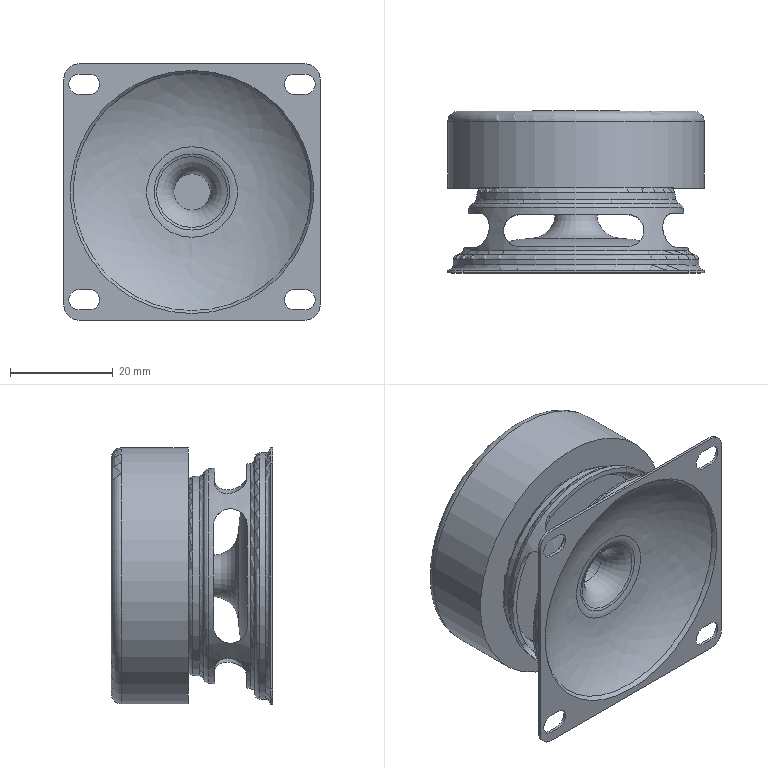Part | STEP file | 2 solids | 77 faces | box 50 x 31.5 x 50 mm | volume 33375 mm3 | plane 31 | cylinder 25 | torus 13 | cone 4 | other 4 | commonest cylinder face diameters 4 x8 6 x4 6.266 x4 6.583 x4 7.086 x1 8.086 x1